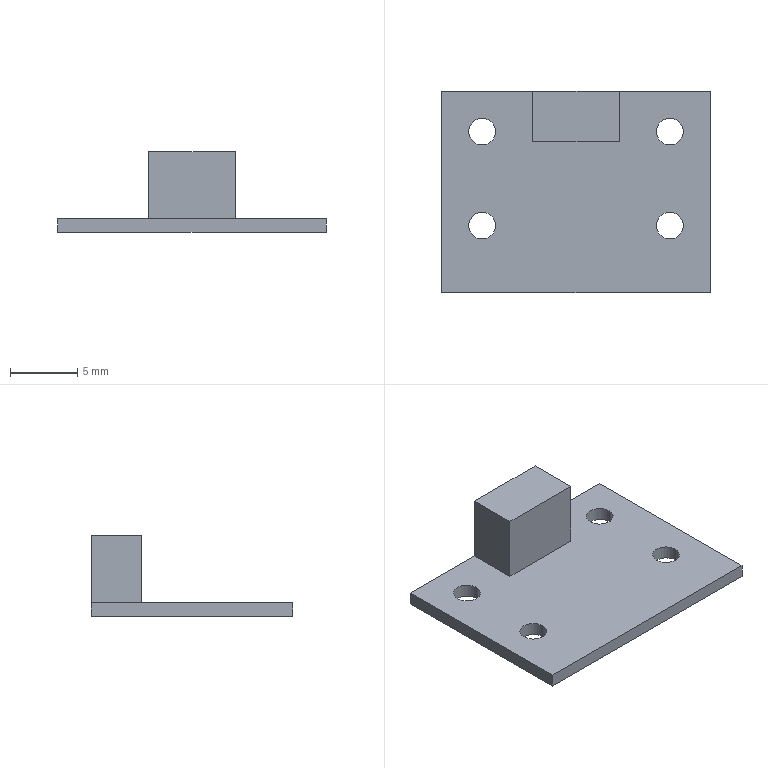Part | SolidWorks | features Extrusion 1, ICE 1 | 1 solid | 18 faces | box 20 x 15 x 6 mm | volume 407.762 mm3 | plane 10 | cylinder 8 | commonest cylinder face diameters 2 x8
STEP:
#1=CARTESIAN_POINT('',(6.,4.5,1.));
#2=VERTEX_POINT('',#1);
#3=CARTESIAN_POINT('',(8.,4.5,1.));
#4=VERTEX_POINT('',#3);
#5=CARTESIAN_POINT('',(7.,4.5,1.));
#6=DIRECTION('',(0.,0.,1.));
#7=DIRECTION('',(1.,0.,0.));
#8=AXIS2_PLACEMENT_3D('',#5,#6,#7);
#9=CIRCLE('',#8,1.);
#10=EDGE_CURVE('',#2,#4,#9,.T.);
#11=ORIENTED_EDGE('',*,*,#10,.T.);
#12=CARTESIAN_POINT('',(8.,4.5,0.));
#13=VERTEX_POINT('',#12);
#14=CARTESIAN_POINT('',(8.,4.5,1.));
#15=DIRECTION('',(0.,0.,-1.));
#16=VECTOR('',#15,1000.);
#17=LINE('',#14,#16);
#18=EDGE_CURVE('',#4,#13,#17,.T.);
#19=ORIENTED_EDGE('',*,*,#18,.T.);
#20=CARTESIAN_POINT('',(6.,4.5,0.));
#21=VERTEX_POINT('',#20);
#22=CARTESIAN_POINT('',(7.,4.5,0.));
#23=DIRECTION('',(0.,0.,1.));
#24=DIRECTION('',(1.,0.,0.));
#25=AXIS2_PLACEMENT_3D('',#22,#23,#24);
#26=CIRCLE('',#25,1.);
#27=EDGE_CURVE('',#21,#13,#26,.T.);
#28=ORIENTED_EDGE('',*,*,#27,.F.);
#29=CARTESIAN_POINT('',(6.,4.5,1.));
#30=DIRECTION('',(0.,0.,-1.));
#31=VECTOR('',#30,1000.);
#32=LINE('',#29,#31);
#33=EDGE_CURVE('',#2,#21,#32,.T.);
#34=ORIENTED_EDGE('',*,*,#33,.F.);
#35=EDGE_LOOP('',(#11,#19,#28,#34));
#36=FACE_OUTER_BOUND('',#35,.T.);
#37=CARTESIAN_POINT('',(7.,4.5,1.));
#38=DIRECTION('',(0.,0.,-1.));
#39=DIRECTION('',(-1.,0.,0.));
#40=AXIS2_PLACEMENT_3D('',#37,#38,#39);
#41=CYLINDRICAL_SURFACE('',#40,1.);
#42=ADVANCED_FACE('',(#36),#41,.F.);
#43=CARTESIAN_POINT('',(6.,-2.5,1.));
#44=VERTEX_POINT('',#43);
#45=CARTESIAN_POINT('',(8.,-2.5,1.));
#46=VERTEX_POINT('',#45);
#47=CARTESIAN_POINT('',(7.,-2.5,1.));
#48=DIRECTION('',(0.,0.,1.));
#49=DIRECTION('',(1.,0.,0.));
#50=AXIS2_PLACEMENT_3D('',#47,#48,#49);
#51=CIRCLE('',#50,1.);
#52=EDGE_CURVE('',#44,#46,#51,.T.);
#53=ORIENTED_EDGE('',*,*,#52,.T.);
#54=CARTESIAN_POINT('',(8.,-2.5,0.));
#55=VERTEX_POINT('',#54);
#56=CARTESIAN_POINT('',(8.,-2.5,1.));
#57=DIRECTION('',(0.,0.,-1.));
#58=VECTOR('',#57,1000.);
#59=LINE('',#56,#58);
#60=EDGE_CURVE('',#46,#55,#59,.T.);
#61=ORIENTED_EDGE('',*,*,#60,.T.);
#62=CARTESIAN_POINT('',(6.,-2.5,0.));
#63=VERTEX_POINT('',#62);
#64=CARTESIAN_POINT('',(7.,-2.5,0.));
#65=DIRECTION('',(0.,0.,1.));
#66=DIRECTION('',(1.,0.,0.));
#67=AXIS2_PLACEMENT_3D('',#64,#65,#66);
#68=CIRCLE('',#67,1.);
#69=EDGE_CURVE('',#63,#55,#68,.T.);
#70=ORIENTED_EDGE('',*,*,#69,.F.);
#71=CARTESIAN_POINT('',(6.,-2.5,1.));
#72=DIRECTION('',(0.,0.,-1.));
#73=VECTOR('',#72,1000.);
#74=LINE('',#71,#73);
#75=EDGE_CURVE('',#44,#63,#74,.T.);
#76=ORIENTED_EDGE('',*,*,#75,.F.);
#77=EDGE_LOOP('',(#53,#61,#70,#76));
#78=FACE_OUTER_BOUND('',#77,.T.);
#79=CARTESIAN_POINT('',(7.,-2.5,1.));
#80=DIRECTION('',(0.,0.,-1.));
#81=DIRECTION('',(-1.,0.,0.));
#82=AXIS2_PLACEMENT_3D('',#79,#80,#81);
#83=CYLINDRICAL_SURFACE('',#82,1.);
#84=ADVANCED_FACE('',(#78),#83,.F.);
#85=CARTESIAN_POINT('',(-8.,-2.5,1.));
#86=VERTEX_POINT('',#85);
#87=CARTESIAN_POINT('',(-6.,-2.5,1.));
#88=VERTEX_POINT('',#87);
#89=CARTESIAN_POINT('',(-7.,-2.5,1.));
#90=DIRECTION('',(0.,0.,1.));
#91=DIRECTION('',(1.,0.,0.));
#92=AXIS2_PLACEMENT_3D('',#89,#90,#91);
#93=CIRCLE('',#92,1.);
#94=EDGE_CURVE('',#86,#88,#93,.T.);
#95=ORIENTED_EDGE('',*,*,#94,.T.);
#96=CARTESIAN_POINT('',(-6.,-2.5,0.));
#97=VERTEX_POINT('',#96);
#98=CARTESIAN_POINT('',(-6.,-2.5,1.));
#99=DIRECTION('',(0.,0.,-1.));
#100=VECTOR('',#99,1000.);
#101=LINE('',#98,#100);
#102=EDGE_CURVE('',#88,#97,#101,.T.);
#103=ORIENTED_EDGE('',*,*,#102,.T.);
#104=CARTESIAN_POINT('',(-8.,-2.5,0.));
#105=VERTEX_POINT('',#104);
#106=CARTESIAN_POINT('',(-7.,-2.5,0.));
#107=DIRECTION('',(0.,0.,1.));
#108=DIRECTION('',(1.,0.,0.));
#109=AXIS2_PLACEMENT_3D('',#106,#107,#108);
#110=CIRCLE('',#109,1.);
#111=EDGE_CURVE('',#105,#97,#110,.T.);
#112=ORIENTED_EDGE('',*,*,#111,.F.);
#113=CARTESIAN_POINT('',(-8.,-2.5,1.));
#114=DIRECTION('',(0.,0.,-1.));
#115=VECTOR('',#114,1000.);
#116=LINE('',#113,#115);
#117=EDGE_CURVE('',#86,#105,#116,.T.);
#118=ORIENTED_EDGE('',*,*,#117,.F.);
#119=EDGE_LOOP('',(#95,#103,#112,#118));
#120=FACE_OUTER_BOUND('',#119,.T.);
#121=CARTESIAN_POINT('',(-7.,-2.5,1.));
#122=DIRECTION('',(0.,0.,-1.));
#123=DIRECTION('',(-1.,0.,0.));
#124=AXIS2_PLACEMENT_3D('',#121,#122,#123);
#125=CYLINDRICAL_SURFACE('',#124,1.);
#126=ADVANCED_FACE('',(#120),#125,.F.);
#127=CARTESIAN_POINT('',(-8.,4.5,1.));
#128=VERTEX_POINT('',#127);
#129=CARTESIAN_POINT('',(-6.,4.5,1.));
#130=VERTEX_POINT('',#129);
#131=CARTESIAN_POINT('',(-7.,4.5,1.));
#132=DIRECTION('',(0.,0.,1.));
#133=DIRECTION('',(1.,0.,0.));
#134=AXIS2_PLACEMENT_3D('',#131,#132,#133);
#135=CIRCLE('',#134,1.);
#136=EDGE_CURVE('',#128,#130,#135,.T.);
#137=ORIENTED_EDGE('',*,*,#136,.T.);
#138=CARTESIAN_POINT('',(-6.,4.5,0.));
#139=VERTEX_POINT('',#138);
#140=CARTESIAN_POINT('',(-6.,4.5,1.));
#141=DIRECTION('',(0.,0.,-1.));
#142=VECTOR('',#141,1000.);
#143=LINE('',#140,#142);
#144=EDGE_CURVE('',#130,#139,#143,.T.);
#145=ORIENTED_EDGE('',*,*,#144,.T.);
#146=CARTESIAN_POINT('',(-8.,4.5,0.));
#147=VERTEX_POINT('',#146);
#148=CARTESIAN_POINT('',(-7.,4.5,0.));
#149=DIRECTION('',(0.,0.,1.));
#150=DIRECTION('',(1.,0.,0.));
#151=AXIS2_PLACEMENT_3D('',#148,#149,#150);
#152=CIRCLE('',#151,1.);
#153=EDGE_CURVE('',#147,#139,#152,.T.);
#154=ORIENTED_EDGE('',*,*,#153,.F.);
#155=CARTESIAN_POINT('',(-8.,4.5,1.));
#156=DIRECTION('',(0.,0.,-1.));
#157=VECTOR('',#156,1000.);
#158=LINE('',#155,#157);
#159=EDGE_CURVE('',#128,#147,#158,.T.);
#160=ORIENTED_EDGE('',*,*,#159,.F.);
#161=EDGE_LOOP('',(#137,#145,#154,#160));
#162=FACE_OUTER_BOUND('',#161,.T.);
#163=CARTESIAN_POINT('',(-7.,4.5,1.));
#164=DIRECTION('',(0.,0.,-1.));
#165=DIRECTION('',(-1.,0.,0.));
#166=AXIS2_PLACEMENT_3D('',#163,#164,#165);
#167=CYLINDRICAL_SURFACE('',#166,1.);
#168=ADVANCED_FACE('',(#162),#167,.F.);
#169=CARTESIAN_POINT('',(3.211,3.753,1.));
#170=VERTEX_POINT('',#169);
#171=CARTESIAN_POINT('',(3.211,7.5,1.));
#172=VERTEX_POINT('',#171);
#173=CARTESIAN_POINT('',(3.211,7.5,1.));
#174=DIRECTION('',(0.,1.,0.));
#175=VECTOR('',#174,1000.);
#176=LINE('',#173,#175);
#177=EDGE_CURVE('',#170,#172,#176,.T.);
#178=ORIENTED_EDGE('',*,*,#177,.F.);
#179=CARTESIAN_POINT('',(-3.211,3.753,1.));
#180=VERTEX_POINT('',#179);
#181=CARTESIAN_POINT('',(-3.211,3.753,1.));
#182=DIRECTION('',(1.,0.,0.));
#183=VECTOR('',#182,1000.);
#184=LINE('',#181,#183);
#185=EDGE_CURVE('',#180,#170,#184,.T.);
#186=ORIENTED_EDGE('',*,*,#185,.F.);
#187=CARTESIAN_POINT('',(-3.211,7.5,1.));
#188=VERTEX_POINT('',#187);
#189=CARTESIAN_POINT('',(-3.211,7.5,1.));
#190=DIRECTION('',(0.,-1.,0.));
#191=VECTOR('',#190,1000.);
#192=LINE('',#189,#191);
#193=EDGE_CURVE('',#188,#180,#192,.T.);
#194=ORIENTED_EDGE('',*,*,#193,.F.);
#195=CARTESIAN_POINT('',(-10.,7.5,1.));
#196=VERTEX_POINT('',#195);
#197=CARTESIAN_POINT('',(-10.,7.5,1.));
#198=DIRECTION('',(-1.,0.,0.));
#199=VECTOR('',#198,1000.);
#200=LINE('',#197,#199);
#201=EDGE_CURVE('',#188,#196,#200,.T.);
#202=ORIENTED_EDGE('',*,*,#201,.T.);
#203=CARTESIAN_POINT('',(-10.,-7.5,1.));
#204=VERTEX_POINT('',#203);
#205=CARTESIAN_POINT('',(-10.,7.5,1.));
#206=DIRECTION('',(0.,-1.,0.));
#207=VECTOR('',#206,1000.);
#208=LINE('',#205,#207);
#209=EDGE_CURVE('',#196,#204,#208,.T.);
#210=ORIENTED_EDGE('',*,*,#209,.T.);
#211=CARTESIAN_POINT('',(10.,-7.5,1.));
#212=VERTEX_POINT('',#211);
#213=CARTESIAN_POINT('',(-10.,-7.5,1.));
#214=DIRECTION('',(1.,0.,0.));
#215=VECTOR('',#214,1000.);
#216=LINE('',#213,#215);
#217=EDGE_CURVE('',#204,#212,#216,.T.);
#218=ORIENTED_EDGE('',*,*,#217,.T.);
#219=CARTESIAN_POINT('',(10.,7.5,1.));
#220=VERTEX_POINT('',#219);
#221=CARTESIAN_POINT('',(10.,7.5,1.));
#222=DIRECTION('',(0.,1.,0.));
#223=VECTOR('',#222,1000.);
#224=LINE('',#221,#223);
#225=EDGE_CURVE('',#212,#220,#224,.T.);
#226=ORIENTED_EDGE('',*,*,#225,.T.);
#227=CARTESIAN_POINT('',(-10.,7.5,1.));
#228=DIRECTION('',(-1.,0.,0.));
#229=VECTOR('',#228,1000.);
#230=LINE('',#227,#229);
#231=EDGE_CURVE('',#220,#172,#230,.T.);
#232=ORIENTED_EDGE('',*,*,#231,.T.);
#233=EDGE_LOOP('',(#178,#186,#194,#202,#210,#218,#226,#232));
#234=FACE_OUTER_BOUND('',#233,.T.);
#235=ORIENTED_EDGE('',*,*,#52,.F.);
#236=CARTESIAN_POINT('',(7.,-2.5,1.));
#237=DIRECTION('',(0.,0.,1.));
#238=DIRECTION('',(1.,0.,0.));
#239=AXIS2_PLACEMENT_3D('',#236,#237,#238);
#240=CIRCLE('',#239,1.);
#241=EDGE_CURVE('',#46,#44,#240,.T.);
#242=ORIENTED_EDGE('',*,*,#241,.F.);
#243=EDGE_LOOP('',(#235,#242));
#244=FACE_BOUND('',#243,.T.);
#245=ORIENTED_EDGE('',*,*,#136,.F.);
#246=CARTESIAN_POINT('',(-7.,4.5,1.));
#247=DIRECTION('',(0.,0.,1.));
#248=DIRECTION('',(1.,0.,0.));
#249=AXIS2_PLACEMENT_3D('',#246,#247,#248);
#250=CIRCLE('',#249,1.);
#251=EDGE_CURVE('',#130,#128,#250,.T.);
#252=ORIENTED_EDGE('',*,*,#251,.F.);
#253=EDGE_LOOP('',(#245,#252));
#254=FACE_BOUND('',#253,.T.);
#255=ORIENTED_EDGE('',*,*,#94,.F.);
#256=CARTESIAN_POINT('',(-7.,-2.5,1.));
#257=DIRECTION('',(0.,0.,1.));
#258=DIRECTION('',(1.,0.,0.));
#259=AXIS2_PLACEMENT_3D('',#256,#257,#258);
#260=CIRCLE('',#259,1.);
#261=EDGE_CURVE('',#88,#86,#260,.T.);
#262=ORIENTED_EDGE('',*,*,#261,.F.);
#263=EDGE_LOOP('',(#255,#262));
#264=FACE_BOUND('',#263,.T.);
#265=ORIENTED_EDGE('',*,*,#10,.F.);
#266=CARTESIAN_POINT('',(7.,4.5,1.));
#267=DIRECTION('',(0.,0.,1.));
#268=DIRECTION('',(1.,0.,0.));
#269=AXIS2_PLACEMENT_3D('',#266,#267,#268);
#270=CIRCLE('',#269,1.);
#271=EDGE_CURVE('',#4,#2,#270,.T.);
#272=ORIENTED_EDGE('',*,*,#271,.F.);
#273=EDGE_LOOP('',(#265,#272));
#274=FACE_BOUND('',#273,.T.);
#275=CARTESIAN_POINT('',(0.,0.,1.));
#276=DIRECTION('',(0.,0.,1.));
#277=DIRECTION('',(1.,0.,0.));
#278=AXIS2_PLACEMENT_3D('',#275,#276,#277);
#279=PLANE('',#278);
#280=ADVANCED_FACE('',(#234,#244,#254,#264,#274),#279,.T.);
#281=CARTESIAN_POINT('',(10.,-7.5,0.));
#282=VERTEX_POINT('',#281);
#283=CARTESIAN_POINT('',(10.,7.5,0.));
#284=VERTEX_POINT('',#283);
#285=CARTESIAN_POINT('',(10.,7.5,0.));
#286=DIRECTION('',(0.,1.,0.));
#287=VECTOR('',#286,1000.);
#288=LINE('',#285,#287);
#289=EDGE_CURVE('',#282,#284,#288,.T.);
#290=ORIENTED_EDGE('',*,*,#289,.F.);
#291=CARTESIAN_POINT('',(-10.,-7.5,0.));
#292=VERTEX_POINT('',#291);
#293=CARTESIAN_POINT('',(-10.,-7.5,0.));
#294=DIRECTION('',(1.,0.,0.));
#295=VECTOR('',#294,1000.);
#296=LINE('',#293,#295);
#297=EDGE_CURVE('',#292,#282,#296,.T.);
#298=ORIENTED_EDGE('',*,*,#297,.F.);
#299=CARTESIAN_POINT('',(-10.,7.5,0.));
#300=VERTEX_POINT('',#299);
#301=CARTESIAN_POINT('',(-10.,7.5,0.));
#302=DIRECTION('',(0.,-1.,0.));
#303=VECTOR('',#302,1000.);
#304=LINE('',#301,#303);
#305=EDGE_CURVE('',#300,#292,#304,.T.);
#306=ORIENTED_EDGE('',*,*,#305,.F.);
#307=CARTESIAN_POINT('',(-10.,7.5,0.));
#308=DIRECTION('',(-1.,0.,0.));
#309=VECTOR('',#308,1000.);
#310=LINE('',#307,#309);
#311=EDGE_CURVE('',#284,#300,#310,.T.);
#312=ORIENTED_EDGE('',*,*,#311,.F.);
#313=EDGE_LOOP('',(#290,#298,#306,#312));
#314=FACE_OUTER_BOUND('',#313,.T.);
#315=ORIENTED_EDGE('',*,*,#153,.T.);
#316=CARTESIAN_POINT('',(-7.,4.5,0.));
#317=DIRECTION('',(0.,0.,1.));
#318=DIRECTION('',(1.,0.,0.));
#319=AXIS2_PLACEMENT_3D('',#316,#317,#318);
#320=CIRCLE('',#319,1.);
#321=EDGE_CURVE('',#139,#147,#320,.T.);
#322=ORIENTED_EDGE('',*,*,#321,.T.);
#323=EDGE_LOOP('',(#315,#322));
#324=FACE_BOUND('',#323,.T.);
#325=ORIENTED_EDGE('',*,*,#111,.T.);
#326=CARTESIAN_POINT('',(-7.,-2.5,0.));
#327=DIRECTION('',(0.,0.,1.));
#328=DIRECTION('',(1.,0.,0.));
#329=AXIS2_PLACEMENT_3D('',#326,#327,#328);
#330=CIRCLE('',#329,1.);
#331=EDGE_CURVE('',#97,#105,#330,.T.);
#332=ORIENTED_EDGE('',*,*,#331,.T.);
#333=EDGE_LOOP('',(#325,#332));
#334=FACE_BOUND('',#333,.T.);
#335=ORIENTED_EDGE('',*,*,#69,.T.);
#336=CARTESIAN_POINT('',(7.,-2.5,0.));
#337=DIRECTION('',(0.,0.,1.));
#338=DIRECTION('',(1.,0.,0.));
#339=AXIS2_PLACEMENT_3D('',#336,#337,#338);
#340=CIRCLE('',#339,1.);
#341=EDGE_CURVE('',#55,#63,#340,.T.);
#342=ORIENTED_EDGE('',*,*,#341,.T.);
#343=EDGE_LOOP('',(#335,#342));
#344=FACE_BOUND('',#343,.T.);
#345=ORIENTED_EDGE('',*,*,#27,.T.);
#346=CARTESIAN_POINT('',(7.,4.5,0.));
#347=DIRECTION('',(0.,0.,1.));
#348=DIRECTION('',(1.,0.,0.));
#349=AXIS2_PLACEMENT_3D('',#346,#347,#348);
#350=CIRCLE('',#349,1.);
#351=EDGE_CURVE('',#13,#21,#350,.T.);
#352=ORIENTED_EDGE('',*,*,#351,.T.);
#353=EDGE_LOOP('',(#345,#352));
#354=FACE_BOUND('',#353,.T.);
#355=CARTESIAN_POINT('',(0.,0.,0.));
#356=DIRECTION('',(0.,0.,1.));
#357=DIRECTION('',(1.,0.,0.));
#358=AXIS2_PLACEMENT_3D('',#355,#356,#357);
#359=PLANE('',#358);
#360=ADVANCED_FACE('',(#314,#324,#334,#344,#354),#359,.F.);
#361=ORIENTED_EDGE('',*,*,#289,.T.);
#362=CARTESIAN_POINT('',(10.,7.5,1.));
#363=DIRECTION('',(0.,0.,-1.));
#364=VECTOR('',#363,1000.);
#365=LINE('',#362,#364);
#366=EDGE_CURVE('',#220,#284,#365,.T.);
#367=ORIENTED_EDGE('',*,*,#366,.F.);
#368=ORIENTED_EDGE('',*,*,#225,.F.);
#369=CARTESIAN_POINT('',(10.,-7.5,1.));
#370=DIRECTION('',(0.,0.,-1.));
#371=VECTOR('',#370,1000.);
#372=LINE('',#369,#371);
#373=EDGE_CURVE('',#212,#282,#372,.T.);
#374=ORIENTED_EDGE('',*,*,#373,.T.);
#375=EDGE_LOOP('',(#361,#367,#368,#374));
#376=FACE_OUTER_BOUND('',#375,.T.);
#377=CARTESIAN_POINT('',(10.,7.5,1.));
#378=DIRECTION('',(-1.,0.,0.));
#379=DIRECTION('',(0.,-1.,0.));
#380=AXIS2_PLACEMENT_3D('',#377,#378,#379);
#381=PLANE('',#380);
#382=ADVANCED_FACE('',(#376),#381,.F.);
#383=ORIENTED_EDGE('',*,*,#311,.T.);
#384=CARTESIAN_POINT('',(-10.,7.5,1.));
#385=DIRECTION('',(0.,0.,-1.));
#386=VECTOR('',#385,1000.);
#387=LINE('',#384,#386);
#388=EDGE_CURVE('',#196,#300,#387,.T.);
#389=ORIENTED_EDGE('',*,*,#388,.F.);
#390=ORIENTED_EDGE('',*,*,#201,.F.);
#391=CARTESIAN_POINT('',(-3.211,7.5,6.));
#392=VERTEX_POINT('',#391);
#393=CARTESIAN_POINT('',(-3.211,7.5,6.));
#394=DIRECTION('',(0.,0.,-1.));
#395=VECTOR('',#394,1000.);
#396=LINE('',#393,#395);
#397=EDGE_CURVE('',#392,#188,#396,.T.);
#398=ORIENTED_EDGE('',*,*,#397,.F.);
#399=CARTESIAN_POINT('',(3.211,7.5,6.));
#400=VERTEX_POINT('',#399);
#401=CARTESIAN_POINT('',(-3.211,7.5,6.));
#402=DIRECTION('',(-1.,0.,0.));
#403=VECTOR('',#402,1000.);
#404=LINE('',#401,#403);
#405=EDGE_CURVE('',#400,#392,#404,.T.);
#406=ORIENTED_EDGE('',*,*,#405,.F.);
#407=CARTESIAN_POINT('',(3.211,7.5,6.));
#408=DIRECTION('',(0.,0.,-1.));
#409=VECTOR('',#408,1000.);
#410=LINE('',#407,#409);
#411=EDGE_CURVE('',#400,#172,#410,.T.);
#412=ORIENTED_EDGE('',*,*,#411,.T.);
#413=ORIENTED_EDGE('',*,*,#231,.F.);
#414=ORIENTED_EDGE('',*,*,#366,.T.);
#415=EDGE_LOOP('',(#383,#389,#390,#398,#406,#412,#413,#414));
#416=FACE_OUTER_BOUND('',#415,.T.);
#417=CARTESIAN_POINT('',(-10.,7.5,1.));
#418=DIRECTION('',(0.,-1.,0.));
#419=DIRECTION('',(1.,0.,0.));
#420=AXIS2_PLACEMENT_3D('',#417,#418,#419);
#421=PLANE('',#420);
#422=ADVANCED_FACE('',(#416),#421,.F.);
#423=ORIENTED_EDGE('',*,*,#305,.T.);
#424=CARTESIAN_POINT('',(-10.,-7.5,1.));
#425=DIRECTION('',(0.,0.,-1.));
#426=VECTOR('',#425,1000.);
#427=LINE('',#424,#426);
#428=EDGE_CURVE('',#204,#292,#427,.T.);
#429=ORIENTED_EDGE('',*,*,#428,.F.);
#430=ORIENTED_EDGE('',*,*,#209,.F.);
#431=ORIENTED_EDGE('',*,*,#388,.T.);
#432=EDGE_LOOP('',(#423,#429,#430,#431));
#433=FACE_OUTER_BOUND('',#432,.T.);
#434=CARTESIAN_POINT('',(-10.,7.5,1.));
#435=DIRECTION('',(1.,0.,0.));
#436=DIRECTION('',(0.,1.,0.));
#437=AXIS2_PLACEMENT_3D('',#434,#435,#436);
#438=PLANE('',#437);
#439=ADVANCED_FACE('',(#433),#438,.F.);
#440=ORIENTED_EDGE('',*,*,#297,.T.);
#441=ORIENTED_EDGE('',*,*,#373,.F.);
#442=ORIENTED_EDGE('',*,*,#217,.F.);
#443=ORIENTED_EDGE('',*,*,#428,.T.);
#444=EDGE_LOOP('',(#440,#441,#442,#443));
#445=FACE_OUTER_BOUND('',#444,.T.);
#446=CARTESIAN_POINT('',(-10.,-7.5,1.));
#447=DIRECTION('',(0.,1.,0.));
#448=DIRECTION('',(0.,0.,1.));
#449=AXIS2_PLACEMENT_3D('',#446,#447,#448);
#450=PLANE('',#449);
#451=ADVANCED_FACE('',(#445),#450,.F.);
#452=ORIENTED_EDGE('',*,*,#144,.F.);
#453=ORIENTED_EDGE('',*,*,#251,.T.);
#454=ORIENTED_EDGE('',*,*,#159,.T.);
#455=ORIENTED_EDGE('',*,*,#321,.F.);
#456=EDGE_LOOP('',(#452,#453,#454,#455));
#457=FACE_OUTER_BOUND('',#456,.T.);
#458=CARTESIAN_POINT('',(-7.,4.5,1.));
#459=DIRECTION('',(0.,0.,-1.));
#460=DIRECTION('',(-1.,0.,0.));
#461=AXIS2_PLACEMENT_3D('',#458,#459,#460);
#462=CYLINDRICAL_SURFACE('',#461,1.);
#463=ADVANCED_FACE('',(#457),#462,.F.);
#464=ORIENTED_EDGE('',*,*,#102,.F.);
#465=ORIENTED_EDGE('',*,*,#261,.T.);
#466=ORIENTED_EDGE('',*,*,#117,.T.);
#467=ORIENTED_EDGE('',*,*,#331,.F.);
#468=EDGE_LOOP('',(#464,#465,#466,#467));
#469=FACE_OUTER_BOUND('',#468,.T.);
#470=CARTESIAN_POINT('',(-7.,-2.5,1.));
#471=DIRECTION('',(0.,0.,-1.));
#472=DIRECTION('',(-1.,0.,0.));
#473=AXIS2_PLACEMENT_3D('',#470,#471,#472);
#474=CYLINDRICAL_SURFACE('',#473,1.);
#475=ADVANCED_FACE('',(#469),#474,.F.);
#476=ORIENTED_EDGE('',*,*,#60,.F.);
#477=ORIENTED_EDGE('',*,*,#241,.T.);
#478=ORIENTED_EDGE('',*,*,#75,.T.);
#479=ORIENTED_EDGE('',*,*,#341,.F.);
#480=EDGE_LOOP('',(#476,#477,#478,#479));
#481=FACE_OUTER_BOUND('',#480,.T.);
#482=CARTESIAN_POINT('',(7.,-2.5,1.));
#483=DIRECTION('',(0.,0.,-1.));
#484=DIRECTION('',(-1.,0.,0.));
#485=AXIS2_PLACEMENT_3D('',#482,#483,#484);
#486=CYLINDRICAL_SURFACE('',#485,1.);
#487=ADVANCED_FACE('',(#481),#486,.F.);
#488=ORIENTED_EDGE('',*,*,#18,.F.);
#489=ORIENTED_EDGE('',*,*,#271,.T.);
#490=ORIENTED_EDGE('',*,*,#33,.T.);
#491=ORIENTED_EDGE('',*,*,#351,.F.);
#492=EDGE_LOOP('',(#488,#489,#490,#491));
#493=FACE_OUTER_BOUND('',#492,.T.);
#494=CARTESIAN_POINT('',(7.,4.5,1.));
#495=DIRECTION('',(0.,0.,-1.));
#496=DIRECTION('',(-1.,0.,0.));
#497=AXIS2_PLACEMENT_3D('',#494,#495,#496);
#498=CYLINDRICAL_SURFACE('',#497,1.);
#499=ADVANCED_FACE('',(#493),#498,.F.);
#500=ORIENTED_EDGE('',*,*,#177,.T.);
#501=ORIENTED_EDGE('',*,*,#411,.F.);
#502=CARTESIAN_POINT('',(3.211,3.753,6.));
#503=VERTEX_POINT('',#502);
#504=CARTESIAN_POINT('',(3.211,7.5,6.));
#505=DIRECTION('',(0.,1.,0.));
#506=VECTOR('',#505,1000.);
#507=LINE('',#504,#506);
#508=EDGE_CURVE('',#503,#400,#507,.T.);
#509=ORIENTED_EDGE('',*,*,#508,.F.);
#510=CARTESIAN_POINT('',(3.211,3.753,6.));
#511=DIRECTION('',(0.,0.,-1.));
#512=VECTOR('',#511,1000.);
#513=LINE('',#510,#512);
#514=EDGE_CURVE('',#503,#170,#513,.T.);
#515=ORIENTED_EDGE('',*,*,#514,.T.);
#516=EDGE_LOOP('',(#500,#501,#509,#515));
#517=FACE_OUTER_BOUND('',#516,.T.);
#518=CARTESIAN_POINT('',(3.211,7.5,6.));
#519=DIRECTION('',(-1.,0.,0.));
#520=DIRECTION('',(0.,-1.,0.));
#521=AXIS2_PLACEMENT_3D('',#518,#519,#520);
#522=PLANE('',#521);
#523=ADVANCED_FACE('',(#517),#522,.F.);
#524=ORIENTED_EDGE('',*,*,#193,.T.);
#525=CARTESIAN_POINT('',(-3.211,3.753,6.));
#526=VERTEX_POINT('',#525);
#527=CARTESIAN_POINT('',(-3.211,3.753,6.));
#528=DIRECTION('',(0.,0.,-1.));
#529=VECTOR('',#528,1000.);
#530=LINE('',#527,#529);
#531=EDGE_CURVE('',#526,#180,#530,.T.);
#532=ORIENTED_EDGE('',*,*,#531,.F.);
#533=CARTESIAN_POINT('',(-3.211,7.5,6.));
#534=DIRECTION('',(0.,-1.,0.));
#535=VECTOR('',#534,1000.);
#536=LINE('',#533,#535);
#537=EDGE_CURVE('',#392,#526,#536,.T.);
#538=ORIENTED_EDGE('',*,*,#537,.F.);
#539=ORIENTED_EDGE('',*,*,#397,.T.);
#540=EDGE_LOOP('',(#524,#532,#538,#539));
#541=FACE_OUTER_BOUND('',#540,.T.);
#542=CARTESIAN_POINT('',(-3.211,7.5,6.));
#543=DIRECTION('',(1.,0.,0.));
#544=DIRECTION('',(0.,1.,0.));
#545=AXIS2_PLACEMENT_3D('',#542,#543,#544);
#546=PLANE('',#545);
#547=ADVANCED_FACE('',(#541),#546,.F.);
#548=ORIENTED_EDGE('',*,*,#185,.T.);
#549=ORIENTED_EDGE('',*,*,#514,.F.);
#550=CARTESIAN_POINT('',(-3.211,3.753,6.));
#551=DIRECTION('',(1.,0.,0.));
#552=VECTOR('',#551,1000.);
#553=LINE('',#550,#552);
#554=EDGE_CURVE('',#526,#503,#553,.T.);
#555=ORIENTED_EDGE('',*,*,#554,.F.);
#556=ORIENTED_EDGE('',*,*,#531,.T.);
#557=EDGE_LOOP('',(#548,#549,#555,#556));
#558=FACE_OUTER_BOUND('',#557,.T.);
#559=CARTESIAN_POINT('',(-3.211,3.753,6.));
#560=DIRECTION('',(0.,1.,0.));
#561=DIRECTION('',(-1.,0.,0.));
#562=AXIS2_PLACEMENT_3D('',#559,#560,#561);
#563=PLANE('',#562);
#564=ADVANCED_FACE('',(#558),#563,.F.);
#565=ORIENTED_EDGE('',*,*,#508,.T.);
#566=ORIENTED_EDGE('',*,*,#405,.T.);
#567=ORIENTED_EDGE('',*,*,#537,.T.);
#568=ORIENTED_EDGE('',*,*,#554,.T.);
#569=EDGE_LOOP('',(#565,#566,#567,#568));
#570=FACE_OUTER_BOUND('',#569,.T.);
#571=CARTESIAN_POINT('',(0.,0.,6.));
#572=DIRECTION('',(0.,0.,1.));
#573=DIRECTION('',(1.,0.,0.));
#574=AXIS2_PLACEMENT_3D('',#571,#572,#573);
#575=PLANE('',#574);
#576=ADVANCED_FACE('',(#570),#575,.T.);
#577=CLOSED_SHELL('',(#42,#84,#126,#168,#280,#360,#382,#422,#439,#451,#463,#475,#487,#499,#523,#547,#564,#576));
#578=MANIFOLD_SOLID_BREP('',#577);
#579=CARTESIAN_POINT('',(0.,0.,0.));
#580=DIRECTION('',(0.,0.,1.));
#581=DIRECTION('',(1.,0.,0.));
#582=AXIS2_PLACEMENT_3D('',#579,#580,#581);
#583=(LENGTH_UNIT()NAMED_UNIT(*)SI_UNIT(.MILLI.,.METRE.));
#584=UNCERTAINTY_MEASURE_WITH_UNIT(LENGTH_MEASURE(0.00001),#583,'','');
#585=(NAMED_UNIT(*)PLANE_ANGLE_UNIT()SI_UNIT($,.RADIAN.));
#586=(NAMED_UNIT(*)SI_UNIT($,.STERADIAN.)SOLID_ANGLE_UNIT());
#587=(GEOMETRIC_REPRESENTATION_CONTEXT(3)GLOBAL_UNCERTAINTY_ASSIGNED_CONTEXT((#584))GLOBAL_UNIT_ASSIGNED_CONTEXT((#583,#585,#586))REPRESENTATION_CONTEXT('',''));
#588=ADVANCED_BREP_SHAPE_REPRESENTATION('',(#578,#582),#587);